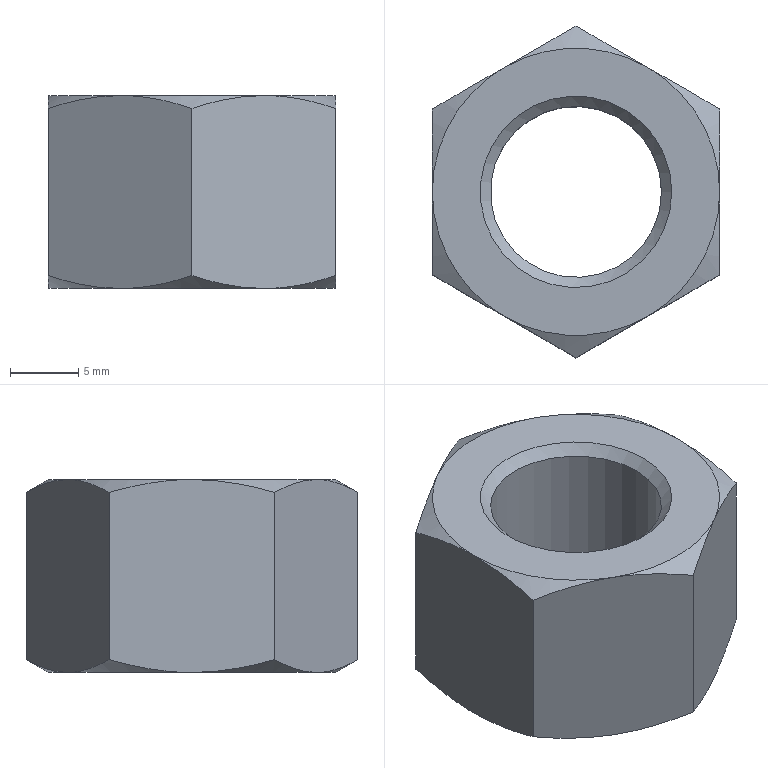Part | NX | features DATUM_CSYS 4, EXTRUDE 3, SKETCH 3, EXTRACT_FACE 2, EXTRACT_STRING 2, HOLE PACKAGE 1, Instance Feature 1, Mirror Feature 1, SIMPLE HOLE 1, SYMBOLIC_THREAD 1 | 1 solid | 23 faces | box 21 x 24.249 x 14.1 mm | volume 3611 mm3 | cone 14 | plane 8 | cylinder 1 | commonest cylinder face diameters 12.5 x1
STEP:
#1=CARTESIAN_POINT('',(-10.5,6.062,13.162));
#2=VERTEX_POINT('',#1);
#3=CARTESIAN_POINT('',(-10.5,6.062,0.9378));
#4=VERTEX_POINT('',#3);
#5=CARTESIAN_POINT('',(-10.5,6.062,14.1));
#6=DIRECTION('',(0.,0.,-1.));
#7=VECTOR('',#6,1000.);
#8=LINE('',#5,#7);
#9=EDGE_CURVE('',#2,#4,#8,.T.);
#10=ORIENTED_EDGE('',*,*,#9,.T.);
#11=CARTESIAN_POINT('',(-10.5,0.,0.));
#12=VERTEX_POINT('',#11);
#13=CARTESIAN_POINT('',(-10.5,0.,0.));
#14=CARTESIAN_POINT('',(-10.5,2.053,0.));
#15=CARTESIAN_POINT('',(-10.5,4.101,0.3717));
#16=CARTESIAN_POINT('',(-10.5,6.062,0.9378));
#17=B_SPLINE_CURVE_WITH_KNOTS('',3,(#13,#14,#15,#16),.UNSPECIFIED.,.F.,.F.,(4,4),(0.01735,0.0235),.UNSPECIFIED.);
#18=EDGE_CURVE('',#4,#12,#17,.F.);
#19=ORIENTED_EDGE('',*,*,#18,.T.);
#20=CARTESIAN_POINT('',(-10.5,-6.062,0.9378));
#21=VERTEX_POINT('',#20);
#22=CARTESIAN_POINT('',(-10.5,-6.062,0.9378));
#23=CARTESIAN_POINT('',(-10.5,-4.088,0.3679));
#24=CARTESIAN_POINT('',(-10.5,-2.051,0.));
#25=CARTESIAN_POINT('',(-10.5,0.,0.));
#26=B_SPLINE_CURVE_WITH_KNOTS('',3,(#22,#23,#24,#25),.UNSPECIFIED.,.F.,.F.,(4,4),(0.01122,0.01735),.UNSPECIFIED.);
#27=EDGE_CURVE('',#12,#21,#26,.F.);
#28=ORIENTED_EDGE('',*,*,#27,.T.);
#29=CARTESIAN_POINT('',(-10.5,-6.062,13.162));
#30=VERTEX_POINT('',#29);
#31=CARTESIAN_POINT('',(-10.5,-6.062,14.1));
#32=DIRECTION('',(0.,0.,-1.));
#33=VECTOR('',#32,1000.);
#34=LINE('',#31,#33);
#35=EDGE_CURVE('',#30,#21,#34,.T.);
#36=ORIENTED_EDGE('',*,*,#35,.F.);
#37=CARTESIAN_POINT('',(-10.5,0.,14.1));
#38=VERTEX_POINT('',#37);
#39=CARTESIAN_POINT('',(-10.5,-6.062,13.162));
#40=CARTESIAN_POINT('',(-10.5,-4.088,13.732));
#41=CARTESIAN_POINT('',(-10.5,-2.051,14.1));
#42=CARTESIAN_POINT('',(-10.5,0.,14.1));
#43=B_SPLINE_CURVE_WITH_KNOTS('',3,(#39,#40,#41,#42),.UNSPECIFIED.,.F.,.F.,(4,4),(0.01122,0.01735),.UNSPECIFIED.);
#44=EDGE_CURVE('',#30,#38,#43,.T.);
#45=ORIENTED_EDGE('',*,*,#44,.T.);
#46=CARTESIAN_POINT('',(-10.5,0.,14.1));
#47=CARTESIAN_POINT('',(-10.5,2.053,14.1));
#48=CARTESIAN_POINT('',(-10.5,4.101,13.728));
#49=CARTESIAN_POINT('',(-10.5,6.062,13.162));
#50=B_SPLINE_CURVE_WITH_KNOTS('',3,(#46,#47,#48,#49),.UNSPECIFIED.,.F.,.F.,(4,4),(0.01735,0.0235),.UNSPECIFIED.);
#51=EDGE_CURVE('',#38,#2,#50,.T.);
#52=ORIENTED_EDGE('',*,*,#51,.T.);
#53=EDGE_LOOP('',(#10,#19,#28,#36,#45,#52));
#54=FACE_BOUND('',#53,.T.);
#55=CARTESIAN_POINT('',(-10.5,6.062,14.1));
#56=DIRECTION('',(1.,0.,0.));
#57=DIRECTION('',(0.,1.,0.));
#58=AXIS2_PLACEMENT_3D('',#55,#56,#57);
#59=PLANE('',#58);
#60=ADVANCED_FACE('',(#54),#59,.F.);
#61=ORIENTED_EDGE('',*,*,#35,.T.);
#62=CARTESIAN_POINT('',(-5.25,-9.093,0.));
#63=VERTEX_POINT('',#62);
#64=CARTESIAN_POINT('',(-10.5,-6.062,0.9378));
#65=CARTESIAN_POINT('',(-8.782,-7.054,0.3653));
#66=CARTESIAN_POINT('',(-7.039,-8.06,0.));
#67=CARTESIAN_POINT('',(-5.25,-9.093,0.));
#68=B_SPLINE_CURVE_WITH_KNOTS('',3,(#64,#65,#66,#67),.UNSPECIFIED.,.F.,.F.,(4,4),(0.000000238,0.006134),.UNSPECIFIED.);
#69=EDGE_CURVE('',#21,#63,#68,.T.);
#70=ORIENTED_EDGE('',*,*,#69,.T.);
#71=CARTESIAN_POINT('',(0.,-12.124,0.9378));
#72=VERTEX_POINT('',#71);
#73=CARTESIAN_POINT('',(-5.25,-9.093,0.));
#74=CARTESIAN_POINT('',(-3.468,-10.122,0.));
#75=CARTESIAN_POINT('',(-1.713,-11.135,0.3667));
#76=CARTESIAN_POINT('',(0.,-12.124,0.9378));
#77=B_SPLINE_CURVE_WITH_KNOTS('',3,(#73,#74,#75,#76),.UNSPECIFIED.,.F.,.F.,(4,4),(0.006134,0.01225),.UNSPECIFIED.);
#78=EDGE_CURVE('',#63,#72,#77,.T.);
#79=ORIENTED_EDGE('',*,*,#78,.T.);
#80=CARTESIAN_POINT('',(0.,-12.124,13.162));
#81=VERTEX_POINT('',#80);
#82=CARTESIAN_POINT('',(0.,-12.124,14.1));
#83=DIRECTION('',(0.,0.,-1.));
#84=VECTOR('',#83,1000.);
#85=LINE('',#82,#84);
#86=EDGE_CURVE('',#81,#72,#85,.T.);
#87=ORIENTED_EDGE('',*,*,#86,.F.);
#88=CARTESIAN_POINT('',(-5.25,-9.093,14.1));
#89=VERTEX_POINT('',#88);
#90=CARTESIAN_POINT('',(-5.25,-9.093,14.1));
#91=CARTESIAN_POINT('',(-3.468,-10.122,14.1));
#92=CARTESIAN_POINT('',(-1.713,-11.135,13.733));
#93=CARTESIAN_POINT('',(0.,-12.124,13.162));
#94=B_SPLINE_CURVE_WITH_KNOTS('',3,(#90,#91,#92,#93),.UNSPECIFIED.,.F.,.F.,(4,4),(0.006134,0.01225),.UNSPECIFIED.);
#95=EDGE_CURVE('',#81,#89,#94,.F.);
#96=ORIENTED_EDGE('',*,*,#95,.T.);
#97=CARTESIAN_POINT('',(-10.5,-6.062,13.162));
#98=CARTESIAN_POINT('',(-8.782,-7.054,13.735));
#99=CARTESIAN_POINT('',(-7.039,-8.06,14.1));
#100=CARTESIAN_POINT('',(-5.25,-9.093,14.1));
#101=B_SPLINE_CURVE_WITH_KNOTS('',3,(#97,#98,#99,#100),.UNSPECIFIED.,.F.,.F.,(4,4),(0.000000238,0.006134),.UNSPECIFIED.);
#102=EDGE_CURVE('',#89,#30,#101,.F.);
#103=ORIENTED_EDGE('',*,*,#102,.T.);
#104=EDGE_LOOP('',(#61,#70,#79,#87,#96,#103));
#105=FACE_BOUND('',#104,.T.);
#106=CARTESIAN_POINT('',(-10.5,-6.062,14.1));
#107=DIRECTION('',(0.5,0.866,0.));
#108=DIRECTION('',(-0.866,0.5,0.));
#109=AXIS2_PLACEMENT_3D('',#106,#107,#108);
#110=PLANE('',#109);
#111=ADVANCED_FACE('',(#105),#110,.F.);
#112=ORIENTED_EDGE('',*,*,#86,.T.);
#113=CARTESIAN_POINT('',(5.25,-9.093,0.));
#114=VERTEX_POINT('',#113);
#115=CARTESIAN_POINT('',(0.,-12.124,0.9378));
#116=CARTESIAN_POINT('',(1.718,-11.133,0.3653));
#117=CARTESIAN_POINT('',(3.461,-10.126,0.));
#118=CARTESIAN_POINT('',(5.25,-9.093,0.));
#119=B_SPLINE_CURVE_WITH_KNOTS('',3,(#115,#116,#117,#118),.UNSPECIFIED.,.F.,.F.,(4,4),(0.000000238,0.006134),.UNSPECIFIED.);
#120=EDGE_CURVE('',#72,#114,#119,.T.);
#121=ORIENTED_EDGE('',*,*,#120,.T.);
#122=CARTESIAN_POINT('',(10.5,-6.062,0.9378));
#123=VERTEX_POINT('',#122);
#124=CARTESIAN_POINT('',(5.25,-9.093,0.));
#125=CARTESIAN_POINT('',(7.032,-8.064,0.));
#126=CARTESIAN_POINT('',(8.787,-7.051,0.3667));
#127=CARTESIAN_POINT('',(10.5,-6.062,0.9378));
#128=B_SPLINE_CURVE_WITH_KNOTS('',3,(#124,#125,#126,#127),.UNSPECIFIED.,.F.,.F.,(4,4),(0.006134,0.01225),.UNSPECIFIED.);
#129=EDGE_CURVE('',#114,#123,#128,.T.);
#130=ORIENTED_EDGE('',*,*,#129,.T.);
#131=CARTESIAN_POINT('',(10.5,-6.062,13.162));
#132=VERTEX_POINT('',#131);
#133=CARTESIAN_POINT('',(10.5,-6.062,14.1));
#134=DIRECTION('',(0.,0.,-1.));
#135=VECTOR('',#134,1000.);
#136=LINE('',#133,#135);
#137=EDGE_CURVE('',#132,#123,#136,.T.);
#138=ORIENTED_EDGE('',*,*,#137,.F.);
#139=CARTESIAN_POINT('',(5.25,-9.093,14.1));
#140=VERTEX_POINT('',#139);
#141=CARTESIAN_POINT('',(5.25,-9.093,14.1));
#142=CARTESIAN_POINT('',(7.032,-8.064,14.1));
#143=CARTESIAN_POINT('',(8.787,-7.051,13.733));
#144=CARTESIAN_POINT('',(10.5,-6.062,13.162));
#145=B_SPLINE_CURVE_WITH_KNOTS('',3,(#141,#142,#143,#144),.UNSPECIFIED.,.F.,.F.,(4,4),(0.006134,0.01225),.UNSPECIFIED.);
#146=EDGE_CURVE('',#132,#140,#145,.F.);
#147=ORIENTED_EDGE('',*,*,#146,.T.);
#148=CARTESIAN_POINT('',(0.,-12.124,13.162));
#149=CARTESIAN_POINT('',(1.718,-11.133,13.735));
#150=CARTESIAN_POINT('',(3.461,-10.126,14.1));
#151=CARTESIAN_POINT('',(5.25,-9.093,14.1));
#152=B_SPLINE_CURVE_WITH_KNOTS('',3,(#148,#149,#150,#151),.UNSPECIFIED.,.F.,.F.,(4,4),(0.000000238,0.006134),.UNSPECIFIED.);
#153=EDGE_CURVE('',#140,#81,#152,.F.);
#154=ORIENTED_EDGE('',*,*,#153,.T.);
#155=EDGE_LOOP('',(#112,#121,#130,#138,#147,#154));
#156=FACE_BOUND('',#155,.T.);
#157=CARTESIAN_POINT('',(0.,-12.124,14.1));
#158=DIRECTION('',(-0.5,0.866,0.));
#159=DIRECTION('',(-0.866,-0.5,0.));
#160=AXIS2_PLACEMENT_3D('',#157,#158,#159);
#161=PLANE('',#160);
#162=ADVANCED_FACE('',(#156),#161,.F.);
#163=ORIENTED_EDGE('',*,*,#137,.T.);
#164=CARTESIAN_POINT('',(10.5,0.,0.));
#165=VERTEX_POINT('',#164);
#166=CARTESIAN_POINT('',(10.5,-6.062,0.9378));
#167=CARTESIAN_POINT('',(10.5,-4.088,0.3679));
#168=CARTESIAN_POINT('',(10.5,-2.051,0.));
#169=CARTESIAN_POINT('',(10.5,0.,0.));
#170=B_SPLINE_CURVE_WITH_KNOTS('',3,(#166,#167,#168,#169),.UNSPECIFIED.,.F.,.F.,(4,4),(0.01122,0.01735),.UNSPECIFIED.);
#171=EDGE_CURVE('',#123,#165,#170,.T.);
#172=ORIENTED_EDGE('',*,*,#171,.T.);
#173=CARTESIAN_POINT('',(10.5,6.062,0.9378));
#174=VERTEX_POINT('',#173);
#175=CARTESIAN_POINT('',(10.5,0.,0.));
#176=CARTESIAN_POINT('',(10.5,2.053,0.));
#177=CARTESIAN_POINT('',(10.5,4.101,0.3717));
#178=CARTESIAN_POINT('',(10.5,6.062,0.9378));
#179=B_SPLINE_CURVE_WITH_KNOTS('',3,(#175,#176,#177,#178),.UNSPECIFIED.,.F.,.F.,(4,4),(0.01735,0.0235),.UNSPECIFIED.);
#180=EDGE_CURVE('',#165,#174,#179,.T.);
#181=ORIENTED_EDGE('',*,*,#180,.T.);
#182=CARTESIAN_POINT('',(10.5,6.062,13.162));
#183=VERTEX_POINT('',#182);
#184=CARTESIAN_POINT('',(10.5,6.062,14.1));
#185=DIRECTION('',(0.,0.,-1.));
#186=VECTOR('',#185,1000.);
#187=LINE('',#184,#186);
#188=EDGE_CURVE('',#183,#174,#187,.T.);
#189=ORIENTED_EDGE('',*,*,#188,.F.);
#190=CARTESIAN_POINT('',(10.5,0.,14.1));
#191=VERTEX_POINT('',#190);
#192=CARTESIAN_POINT('',(10.5,0.,14.1));
#193=CARTESIAN_POINT('',(10.5,2.053,14.1));
#194=CARTESIAN_POINT('',(10.5,4.101,13.728));
#195=CARTESIAN_POINT('',(10.5,6.062,13.162));
#196=B_SPLINE_CURVE_WITH_KNOTS('',3,(#192,#193,#194,#195),.UNSPECIFIED.,.F.,.F.,(4,4),(0.01735,0.0235),.UNSPECIFIED.);
#197=EDGE_CURVE('',#183,#191,#196,.F.);
#198=ORIENTED_EDGE('',*,*,#197,.T.);
#199=CARTESIAN_POINT('',(10.5,-6.062,13.162));
#200=CARTESIAN_POINT('',(10.5,-4.088,13.732));
#201=CARTESIAN_POINT('',(10.5,-2.051,14.1));
#202=CARTESIAN_POINT('',(10.5,0.,14.1));
#203=B_SPLINE_CURVE_WITH_KNOTS('',3,(#199,#200,#201,#202),.UNSPECIFIED.,.F.,.F.,(4,4),(0.01122,0.01735),.UNSPECIFIED.);
#204=EDGE_CURVE('',#191,#132,#203,.F.);
#205=ORIENTED_EDGE('',*,*,#204,.T.);
#206=EDGE_LOOP('',(#163,#172,#181,#189,#198,#205));
#207=FACE_BOUND('',#206,.T.);
#208=CARTESIAN_POINT('',(10.5,-6.062,14.1));
#209=DIRECTION('',(-1.,0.,0.));
#210=DIRECTION('',(0.,-1.,0.));
#211=AXIS2_PLACEMENT_3D('',#208,#209,#210);
#212=PLANE('',#211);
#213=ADVANCED_FACE('',(#207),#212,.F.);
#214=ORIENTED_EDGE('',*,*,#188,.T.);
#215=CARTESIAN_POINT('',(5.25,9.093,0.));
#216=VERTEX_POINT('',#215);
#217=CARTESIAN_POINT('',(10.5,6.062,0.9378));
#218=CARTESIAN_POINT('',(8.782,7.054,0.3653));
#219=CARTESIAN_POINT('',(7.039,8.06,0.));
#220=CARTESIAN_POINT('',(5.25,9.093,0.));
#221=B_SPLINE_CURVE_WITH_KNOTS('',3,(#217,#218,#219,#220),.UNSPECIFIED.,.F.,.F.,(4,4),(0.000000238,0.006134),.UNSPECIFIED.);
#222=EDGE_CURVE('',#174,#216,#221,.T.);
#223=ORIENTED_EDGE('',*,*,#222,.T.);
#224=CARTESIAN_POINT('',(0.,12.124,0.9378));
#225=VERTEX_POINT('',#224);
#226=CARTESIAN_POINT('',(5.25,9.093,0.));
#227=CARTESIAN_POINT('',(3.468,10.122,0.));
#228=CARTESIAN_POINT('',(1.713,11.135,0.3667));
#229=CARTESIAN_POINT('',(0.,12.124,0.9378));
#230=B_SPLINE_CURVE_WITH_KNOTS('',3,(#226,#227,#228,#229),.UNSPECIFIED.,.F.,.F.,(4,4),(0.006134,0.01225),.UNSPECIFIED.);
#231=EDGE_CURVE('',#216,#225,#230,.T.);
#232=ORIENTED_EDGE('',*,*,#231,.T.);
#233=CARTESIAN_POINT('',(0.,12.124,13.162));
#234=VERTEX_POINT('',#233);
#235=CARTESIAN_POINT('',(0.,12.124,14.1));
#236=DIRECTION('',(0.,0.,-1.));
#237=VECTOR('',#236,1000.);
#238=LINE('',#235,#237);
#239=EDGE_CURVE('',#234,#225,#238,.T.);
#240=ORIENTED_EDGE('',*,*,#239,.F.);
#241=CARTESIAN_POINT('',(5.25,9.093,14.1));
#242=VERTEX_POINT('',#241);
#243=CARTESIAN_POINT('',(5.25,9.093,14.1));
#244=CARTESIAN_POINT('',(3.468,10.122,14.1));
#245=CARTESIAN_POINT('',(1.713,11.135,13.733));
#246=CARTESIAN_POINT('',(0.,12.124,13.162));
#247=B_SPLINE_CURVE_WITH_KNOTS('',3,(#243,#244,#245,#246),.UNSPECIFIED.,.F.,.F.,(4,4),(0.006134,0.01225),.UNSPECIFIED.);
#248=EDGE_CURVE('',#234,#242,#247,.F.);
#249=ORIENTED_EDGE('',*,*,#248,.T.);
#250=CARTESIAN_POINT('',(10.5,6.062,13.162));
#251=CARTESIAN_POINT('',(8.782,7.054,13.735));
#252=CARTESIAN_POINT('',(7.039,8.06,14.1));
#253=CARTESIAN_POINT('',(5.25,9.093,14.1));
#254=B_SPLINE_CURVE_WITH_KNOTS('',3,(#250,#251,#252,#253),.UNSPECIFIED.,.F.,.F.,(4,4),(0.000000238,0.006134),.UNSPECIFIED.);
#255=EDGE_CURVE('',#242,#183,#254,.F.);
#256=ORIENTED_EDGE('',*,*,#255,.T.);
#257=EDGE_LOOP('',(#214,#223,#232,#240,#249,#256));
#258=FACE_BOUND('',#257,.T.);
#259=CARTESIAN_POINT('',(10.5,6.062,14.1));
#260=DIRECTION('',(-0.5,-0.866,0.));
#261=DIRECTION('',(0.866,-0.5,0.));
#262=AXIS2_PLACEMENT_3D('',#259,#260,#261);
#263=PLANE('',#262);
#264=ADVANCED_FACE('',(#258),#263,.F.);
#265=ORIENTED_EDGE('',*,*,#239,.T.);
#266=CARTESIAN_POINT('',(-5.25,9.093,0.));
#267=VERTEX_POINT('',#266);
#268=CARTESIAN_POINT('',(0.,12.124,0.9378));
#269=CARTESIAN_POINT('',(-1.718,11.133,0.3653));
#270=CARTESIAN_POINT('',(-3.461,10.126,0.));
#271=CARTESIAN_POINT('',(-5.25,9.093,0.));
#272=B_SPLINE_CURVE_WITH_KNOTS('',3,(#268,#269,#270,#271),.UNSPECIFIED.,.F.,.F.,(4,4),(0.000000238,0.006134),.UNSPECIFIED.);
#273=EDGE_CURVE('',#225,#267,#272,.T.);
#274=ORIENTED_EDGE('',*,*,#273,.T.);
#275=CARTESIAN_POINT('',(-5.25,9.093,0.));
#276=CARTESIAN_POINT('',(-7.032,8.064,0.));
#277=CARTESIAN_POINT('',(-8.787,7.051,0.3667));
#278=CARTESIAN_POINT('',(-10.5,6.062,0.9378));
#279=B_SPLINE_CURVE_WITH_KNOTS('',3,(#275,#276,#277,#278),.UNSPECIFIED.,.F.,.F.,(4,4),(0.006134,0.01225),.UNSPECIFIED.);
#280=EDGE_CURVE('',#267,#4,#279,.T.);
#281=ORIENTED_EDGE('',*,*,#280,.T.);
#282=ORIENTED_EDGE('',*,*,#9,.F.);
#283=CARTESIAN_POINT('',(-5.25,9.093,14.1));
#284=VERTEX_POINT('',#283);
#285=CARTESIAN_POINT('',(-5.25,9.093,14.1));
#286=CARTESIAN_POINT('',(-7.032,8.064,14.1));
#287=CARTESIAN_POINT('',(-8.787,7.051,13.733));
#288=CARTESIAN_POINT('',(-10.5,6.062,13.162));
#289=B_SPLINE_CURVE_WITH_KNOTS('',3,(#285,#286,#287,#288),.UNSPECIFIED.,.F.,.F.,(4,4),(0.006134,0.01225),.UNSPECIFIED.);
#290=EDGE_CURVE('',#2,#284,#289,.F.);
#291=ORIENTED_EDGE('',*,*,#290,.T.);
#292=CARTESIAN_POINT('',(0.,12.124,13.162));
#293=CARTESIAN_POINT('',(-1.718,11.133,13.735));
#294=CARTESIAN_POINT('',(-3.461,10.126,14.1));
#295=CARTESIAN_POINT('',(-5.25,9.093,14.1));
#296=B_SPLINE_CURVE_WITH_KNOTS('',3,(#292,#293,#294,#295),.UNSPECIFIED.,.F.,.F.,(4,4),(0.000000238,0.006134),.UNSPECIFIED.);
#297=EDGE_CURVE('',#284,#234,#296,.F.);
#298=ORIENTED_EDGE('',*,*,#297,.T.);
#299=EDGE_LOOP('',(#265,#274,#281,#282,#291,#298));
#300=FACE_BOUND('',#299,.T.);
#301=CARTESIAN_POINT('',(0.,12.124,14.1));
#302=DIRECTION('',(0.5,-0.866,0.));
#303=DIRECTION('',(0.866,0.5,0.));
#304=AXIS2_PLACEMENT_3D('',#301,#302,#303);
#305=PLANE('',#304);
#306=ADVANCED_FACE('',(#300),#305,.F.);
#307=ORIENTED_EDGE('',*,*,#290,.F.);
#308=ORIENTED_EDGE('',*,*,#51,.F.);
#309=CARTESIAN_POINT('',(0.,0.,14.1));
#310=DIRECTION('',(0.,0.,1.));
#311=DIRECTION('',(0.,1.,0.));
#312=AXIS2_PLACEMENT_3D('',#309,#310,#311);
#313=CIRCLE('',#312,10.5);
#314=EDGE_CURVE('',#38,#284,#313,.F.);
#315=ORIENTED_EDGE('',*,*,#314,.T.);
#316=EDGE_LOOP('',(#307,#308,#315));
#317=FACE_BOUND('',#316,.T.);
#318=CARTESIAN_POINT('',(0.,0.,14.1));
#319=DIRECTION('',(0.,0.,-1.));
#320=DIRECTION('',(0.,1.,0.));
#321=AXIS2_PLACEMENT_3D('',#318,#319,#320);
#322=CONICAL_SURFACE('',#321,10.5,1.047);
#323=ADVANCED_FACE('',(#317),#322,.T.);
#324=CARTESIAN_POINT('',(0.,0.,14.1));
#325=DIRECTION('',(0.,0.,1.));
#326=DIRECTION('',(0.,1.,0.));
#327=AXIS2_PLACEMENT_3D('',#324,#325,#326);
#328=CIRCLE('',#327,10.5);
#329=EDGE_CURVE('',#284,#242,#328,.F.);
#330=ORIENTED_EDGE('',*,*,#329,.T.);
#331=ORIENTED_EDGE('',*,*,#248,.F.);
#332=ORIENTED_EDGE('',*,*,#297,.F.);
#333=EDGE_LOOP('',(#330,#331,#332));
#334=FACE_BOUND('',#333,.T.);
#335=CARTESIAN_POINT('',(0.,0.,14.1));
#336=DIRECTION('',(0.,0.,-1.));
#337=DIRECTION('',(0.,1.,0.));
#338=AXIS2_PLACEMENT_3D('',#335,#336,#337);
#339=CONICAL_SURFACE('',#338,10.5,1.047);
#340=ADVANCED_FACE('',(#334),#339,.T.);
#341=CARTESIAN_POINT('',(0.,0.,14.1));
#342=DIRECTION('',(0.,0.,1.));
#343=DIRECTION('',(0.,1.,0.));
#344=AXIS2_PLACEMENT_3D('',#341,#342,#343);
#345=CIRCLE('',#344,10.5);
#346=EDGE_CURVE('',#242,#191,#345,.F.);
#347=ORIENTED_EDGE('',*,*,#346,.T.);
#348=ORIENTED_EDGE('',*,*,#197,.F.);
#349=ORIENTED_EDGE('',*,*,#255,.F.);
#350=EDGE_LOOP('',(#347,#348,#349));
#351=FACE_BOUND('',#350,.T.);
#352=CARTESIAN_POINT('',(0.,0.,14.1));
#353=DIRECTION('',(0.,0.,-1.));
#354=DIRECTION('',(0.,1.,0.));
#355=AXIS2_PLACEMENT_3D('',#352,#353,#354);
#356=CONICAL_SURFACE('',#355,10.5,1.047);
#357=ADVANCED_FACE('',(#351),#356,.T.);
#358=CARTESIAN_POINT('',(0.,0.,14.1));
#359=DIRECTION('',(0.,0.,1.));
#360=DIRECTION('',(0.,1.,0.));
#361=AXIS2_PLACEMENT_3D('',#358,#359,#360);
#362=CIRCLE('',#361,10.5);
#363=EDGE_CURVE('',#191,#140,#362,.F.);
#364=ORIENTED_EDGE('',*,*,#363,.T.);
#365=ORIENTED_EDGE('',*,*,#146,.F.);
#366=ORIENTED_EDGE('',*,*,#204,.F.);
#367=EDGE_LOOP('',(#364,#365,#366));
#368=FACE_BOUND('',#367,.T.);
#369=CARTESIAN_POINT('',(0.,0.,14.1));
#370=DIRECTION('',(0.,0.,-1.));
#371=DIRECTION('',(0.,1.,0.));
#372=AXIS2_PLACEMENT_3D('',#369,#370,#371);
#373=CONICAL_SURFACE('',#372,10.5,1.047);
#374=ADVANCED_FACE('',(#368),#373,.T.);
#375=CARTESIAN_POINT('',(0.,0.,14.1));
#376=DIRECTION('',(0.,0.,1.));
#377=DIRECTION('',(0.,1.,0.));
#378=AXIS2_PLACEMENT_3D('',#375,#376,#377);
#379=CIRCLE('',#378,10.5);
#380=EDGE_CURVE('',#140,#89,#379,.F.);
#381=ORIENTED_EDGE('',*,*,#380,.T.);
#382=ORIENTED_EDGE('',*,*,#95,.F.);
#383=ORIENTED_EDGE('',*,*,#153,.F.);
#384=EDGE_LOOP('',(#381,#382,#383));
#385=FACE_BOUND('',#384,.T.);
#386=CARTESIAN_POINT('',(0.,0.,14.1));
#387=DIRECTION('',(0.,0.,-1.));
#388=DIRECTION('',(0.,1.,0.));
#389=AXIS2_PLACEMENT_3D('',#386,#387,#388);
#390=CONICAL_SURFACE('',#389,10.5,1.047);
#391=ADVANCED_FACE('',(#385),#390,.T.);
#392=CARTESIAN_POINT('',(0.,0.,14.1));
#393=DIRECTION('',(0.,0.,1.));
#394=DIRECTION('',(0.,1.,0.));
#395=AXIS2_PLACEMENT_3D('',#392,#393,#394);
#396=CIRCLE('',#395,10.5);
#397=EDGE_CURVE('',#89,#38,#396,.F.);
#398=ORIENTED_EDGE('',*,*,#397,.T.);
#399=ORIENTED_EDGE('',*,*,#44,.F.);
#400=ORIENTED_EDGE('',*,*,#102,.F.);
#401=EDGE_LOOP('',(#398,#399,#400));
#402=FACE_BOUND('',#401,.T.);
#403=CARTESIAN_POINT('',(0.,0.,14.1));
#404=DIRECTION('',(0.,0.,-1.));
#405=DIRECTION('',(0.,1.,0.));
#406=AXIS2_PLACEMENT_3D('',#403,#404,#405);
#407=CONICAL_SURFACE('',#406,10.5,1.047);
#408=ADVANCED_FACE('',(#402),#407,.T.);
#409=CARTESIAN_POINT('',(7.,0.,14.1));
#410=VERTEX_POINT('',#409);
#411=CARTESIAN_POINT('',(0.,0.,14.1));
#412=DIRECTION('',(0.,0.,1.));
#413=DIRECTION('',(1.,0.,0.));
#414=AXIS2_PLACEMENT_3D('',#411,#412,#413);
#415=CIRCLE('',#414,7.);
#416=EDGE_CURVE('',#410,#410,#415,.F.);
#417=ORIENTED_EDGE('',*,*,#416,.T.);
#418=EDGE_LOOP('',(#417));
#419=FACE_BOUND('',#418,.T.);
#420=ORIENTED_EDGE('',*,*,#329,.F.);
#421=ORIENTED_EDGE('',*,*,#314,.F.);
#422=ORIENTED_EDGE('',*,*,#397,.F.);
#423=ORIENTED_EDGE('',*,*,#380,.F.);
#424=ORIENTED_EDGE('',*,*,#363,.F.);
#425=ORIENTED_EDGE('',*,*,#346,.F.);
#426=EDGE_LOOP('',(#420,#421,#422,#423,#424,#425));
#427=FACE_BOUND('',#426,.T.);
#428=CARTESIAN_POINT('',(0.,0.,14.1));
#429=DIRECTION('',(0.,0.,1.));
#430=DIRECTION('',(1.,0.,0.));
#431=AXIS2_PLACEMENT_3D('',#428,#429,#430);
#432=PLANE('',#431);
#433=ADVANCED_FACE('',(#419,#427),#432,.T.);
#434=ORIENTED_EDGE('',*,*,#18,.F.);
#435=ORIENTED_EDGE('',*,*,#280,.F.);
#436=CARTESIAN_POINT('',(0.,0.,0.));
#437=DIRECTION('',(0.,0.,1.));
#438=DIRECTION('',(0.,1.,0.));
#439=AXIS2_PLACEMENT_3D('',#436,#437,#438);
#440=CIRCLE('',#439,10.5);
#441=EDGE_CURVE('',#267,#12,#440,.T.);
#442=ORIENTED_EDGE('',*,*,#441,.T.);
#443=EDGE_LOOP('',(#434,#435,#442));
#444=FACE_BOUND('',#443,.T.);
#445=CARTESIAN_POINT('',(0.,0.,0.));
#446=DIRECTION('',(0.,0.,1.));
#447=DIRECTION('',(0.,1.,0.));
#448=AXIS2_PLACEMENT_3D('',#445,#446,#447);
#449=CONICAL_SURFACE('',#448,10.5,1.047);
#450=ADVANCED_FACE('',(#444),#449,.T.);
#451=ORIENTED_EDGE('',*,*,#231,.F.);
#452=CARTESIAN_POINT('',(0.,0.,0.));
#453=DIRECTION('',(0.,0.,1.));
#454=DIRECTION('',(0.,1.,0.));
#455=AXIS2_PLACEMENT_3D('',#452,#453,#454);
#456=CIRCLE('',#455,10.5);
#457=EDGE_CURVE('',#216,#267,#456,.T.);
#458=ORIENTED_EDGE('',*,*,#457,.T.);
#459=ORIENTED_EDGE('',*,*,#273,.F.);
#460=EDGE_LOOP('',(#451,#458,#459));
#461=FACE_BOUND('',#460,.T.);
#462=CARTESIAN_POINT('',(0.,0.,0.));
#463=DIRECTION('',(0.,0.,1.));
#464=DIRECTION('',(0.,1.,0.));
#465=AXIS2_PLACEMENT_3D('',#462,#463,#464);
#466=CONICAL_SURFACE('',#465,10.5,1.047);
#467=ADVANCED_FACE('',(#461),#466,.T.);
#468=ORIENTED_EDGE('',*,*,#180,.F.);
#469=CARTESIAN_POINT('',(0.,0.,0.));
#470=DIRECTION('',(0.,0.,1.));
#471=DIRECTION('',(0.,1.,0.));
#472=AXIS2_PLACEMENT_3D('',#469,#470,#471);
#473=CIRCLE('',#472,10.5);
#474=EDGE_CURVE('',#165,#216,#473,.T.);
#475=ORIENTED_EDGE('',*,*,#474,.T.);
#476=ORIENTED_EDGE('',*,*,#222,.F.);
#477=EDGE_LOOP('',(#468,#475,#476));
#478=FACE_BOUND('',#477,.T.);
#479=CARTESIAN_POINT('',(0.,0.,0.));
#480=DIRECTION('',(0.,0.,1.));
#481=DIRECTION('',(0.,1.,0.));
#482=AXIS2_PLACEMENT_3D('',#479,#480,#481);
#483=CONICAL_SURFACE('',#482,10.5,1.047);
#484=ADVANCED_FACE('',(#478),#483,.T.);
#485=ORIENTED_EDGE('',*,*,#129,.F.);
#486=CARTESIAN_POINT('',(0.,0.,0.));
#487=DIRECTION('',(0.,0.,1.));
#488=DIRECTION('',(0.,1.,0.));
#489=AXIS2_PLACEMENT_3D('',#486,#487,#488);
#490=CIRCLE('',#489,10.5);
#491=EDGE_CURVE('',#114,#165,#490,.T.);
#492=ORIENTED_EDGE('',*,*,#491,.T.);
#493=ORIENTED_EDGE('',*,*,#171,.F.);
#494=EDGE_LOOP('',(#485,#492,#493));
#495=FACE_BOUND('',#494,.T.);
#496=CARTESIAN_POINT('',(0.,0.,0.));
#497=DIRECTION('',(0.,0.,1.));
#498=DIRECTION('',(0.,1.,0.));
#499=AXIS2_PLACEMENT_3D('',#496,#497,#498);
#500=CONICAL_SURFACE('',#499,10.5,1.047);
#501=ADVANCED_FACE('',(#495),#500,.T.);
#502=ORIENTED_EDGE('',*,*,#78,.F.);
#503=CARTESIAN_POINT('',(0.,0.,0.));
#504=DIRECTION('',(0.,0.,1.));
#505=DIRECTION('',(0.,1.,0.));
#506=AXIS2_PLACEMENT_3D('',#503,#504,#505);
#507=CIRCLE('',#506,10.5);
#508=EDGE_CURVE('',#63,#114,#507,.T.);
#509=ORIENTED_EDGE('',*,*,#508,.T.);
#510=ORIENTED_EDGE('',*,*,#120,.F.);
#511=EDGE_LOOP('',(#502,#509,#510));
#512=FACE_BOUND('',#511,.T.);
#513=CARTESIAN_POINT('',(0.,0.,0.));
#514=DIRECTION('',(0.,0.,1.));
#515=DIRECTION('',(0.,1.,0.));
#516=AXIS2_PLACEMENT_3D('',#513,#514,#515);
#517=CONICAL_SURFACE('',#516,10.5,1.047);
#518=ADVANCED_FACE('',(#512),#517,.T.);
#519=ORIENTED_EDGE('',*,*,#27,.F.);
#520=CARTESIAN_POINT('',(0.,0.,0.));
#521=DIRECTION('',(0.,0.,1.));
#522=DIRECTION('',(0.,1.,0.));
#523=AXIS2_PLACEMENT_3D('',#520,#521,#522);
#524=CIRCLE('',#523,10.5);
#525=EDGE_CURVE('',#12,#63,#524,.T.);
#526=ORIENTED_EDGE('',*,*,#525,.T.);
#527=ORIENTED_EDGE('',*,*,#69,.F.);
#528=EDGE_LOOP('',(#519,#526,#527));
#529=FACE_BOUND('',#528,.T.);
#530=CARTESIAN_POINT('',(0.,0.,0.));
#531=DIRECTION('',(0.,0.,1.));
#532=DIRECTION('',(0.,1.,0.));
#533=AXIS2_PLACEMENT_3D('',#530,#531,#532);
#534=CONICAL_SURFACE('',#533,10.5,1.047);
#535=ADVANCED_FACE('',(#529),#534,.T.);
#536=CARTESIAN_POINT('',(7.,0.,0.));
#537=VERTEX_POINT('',#536);
#538=CARTESIAN_POINT('',(0.,0.,0.));
#539=DIRECTION('',(0.,0.,1.));
#540=DIRECTION('',(1.,0.,0.));
#541=AXIS2_PLACEMENT_3D('',#538,#539,#540);
#542=CIRCLE('',#541,7.);
#543=EDGE_CURVE('',#537,#537,#542,.T.);
#544=ORIENTED_EDGE('',*,*,#543,.T.);
#545=EDGE_LOOP('',(#544));
#546=FACE_BOUND('',#545,.T.);
#547=ORIENTED_EDGE('',*,*,#441,.F.);
#548=ORIENTED_EDGE('',*,*,#457,.F.);
#549=ORIENTED_EDGE('',*,*,#474,.F.);
#550=ORIENTED_EDGE('',*,*,#491,.F.);
#551=ORIENTED_EDGE('',*,*,#508,.F.);
#552=ORIENTED_EDGE('',*,*,#525,.F.);
#553=EDGE_LOOP('',(#547,#548,#549,#550,#551,#552));
#554=FACE_BOUND('',#553,.T.);
#555=CARTESIAN_POINT('',(0.,0.,0.));
#556=DIRECTION('',(0.,0.,1.));
#557=DIRECTION('',(1.,0.,0.));
#558=AXIS2_PLACEMENT_3D('',#555,#556,#557);
#559=PLANE('',#558);
#560=ADVANCED_FACE('',(#546,#554),#559,.F.);
#561=CARTESIAN_POINT('',(6.25,0.,0.75));
#562=VERTEX_POINT('',#561);
#563=CARTESIAN_POINT('',(0.,0.,0.75));
#564=DIRECTION('',(0.,0.,1.));
#565=DIRECTION('',(1.,0.,0.));
#566=AXIS2_PLACEMENT_3D('',#563,#564,#565);
#567=CIRCLE('',#566,6.25);
#568=EDGE_CURVE('',#562,#562,#567,.F.);
#569=ORIENTED_EDGE('',*,*,#568,.T.);
#570=EDGE_LOOP('',(#569));
#571=FACE_BOUND('',#570,.T.);
#572=CARTESIAN_POINT('',(6.25,0.,13.35));
#573=VERTEX_POINT('',#572);
#574=CARTESIAN_POINT('',(0.,0.,13.35));
#575=DIRECTION('',(0.,0.,1.));
#576=DIRECTION('',(1.,0.,0.));
#577=AXIS2_PLACEMENT_3D('',#574,#575,#576);
#578=CIRCLE('',#577,6.25);
#579=EDGE_CURVE('',#573,#573,#578,.T.);
#580=ORIENTED_EDGE('',*,*,#579,.T.);
#581=EDGE_LOOP('',(#580));
#582=FACE_BOUND('',#581,.T.);
#583=CARTESIAN_POINT('',(0.,0.,14.1));
#584=DIRECTION('',(0.,0.,-1.));
#585=DIRECTION('',(-1.,0.,0.));
#586=AXIS2_PLACEMENT_3D('',#583,#584,#585);
#587=CYLINDRICAL_SURFACE('',#586,6.25);
#588=ADVANCED_FACE('',(#571,#582),#587,.F.);
#589=ORIENTED_EDGE('',*,*,#579,.F.);
#590=EDGE_LOOP('',(#589));
#591=FACE_BOUND('',#590,.T.);
#592=ORIENTED_EDGE('',*,*,#416,.F.);
#593=EDGE_LOOP('',(#592));
#594=FACE_BOUND('',#593,.T.);
#595=CARTESIAN_POINT('',(0.,0.,14.1));
#596=DIRECTION('',(0.,0.,1.));
#597=DIRECTION('',(1.,0.,0.));
#598=AXIS2_PLACEMENT_3D('',#595,#596,#597);
#599=CONICAL_SURFACE('',#598,7.,0.7854);
#600=ADVANCED_FACE('',(#591,#594),#599,.F.);
#601=ORIENTED_EDGE('',*,*,#568,.F.);
#602=EDGE_LOOP('',(#601));
#603=FACE_BOUND('',#602,.T.);
#604=ORIENTED_EDGE('',*,*,#543,.F.);
#605=EDGE_LOOP('',(#604));
#606=FACE_BOUND('',#605,.T.);
#607=CARTESIAN_POINT('',(0.,0.,0.));
#608=DIRECTION('',(0.,0.,-1.));
#609=DIRECTION('',(-1.,0.,0.));
#610=AXIS2_PLACEMENT_3D('',#607,#608,#609);
#611=CONICAL_SURFACE('',#610,7.,0.7854);
#612=ADVANCED_FACE('',(#603,#606),#611,.F.);
#613=CLOSED_SHELL('',(#60,#111,#162,#213,#264,#306,#323,#340,#357,#374,#391,#408,#433,#450,#467,#484,#501,#518,#535,#560,#588,#600,#612));
#614=MANIFOLD_SOLID_BREP('',#613);
#615=(LENGTH_UNIT()NAMED_UNIT(*)SI_UNIT(.MILLI.,.METRE.));
#616=UNCERTAINTY_MEASURE_WITH_UNIT(LENGTH_MEASURE(0.0508),#615,'','');
#617=(NAMED_UNIT(*)PLANE_ANGLE_UNIT()SI_UNIT($,.RADIAN.));
#618=(NAMED_UNIT(*)SI_UNIT($,.STERADIAN.)SOLID_ANGLE_UNIT());
#619=(GEOMETRIC_REPRESENTATION_CONTEXT(3)GLOBAL_UNCERTAINTY_ASSIGNED_CONTEXT((#616))GLOBAL_UNIT_ASSIGNED_CONTEXT((#615,#617,#618))REPRESENTATION_CONTEXT('',''));
#620=ADVANCED_BREP_SHAPE_REPRESENTATION('',(#614),#619);